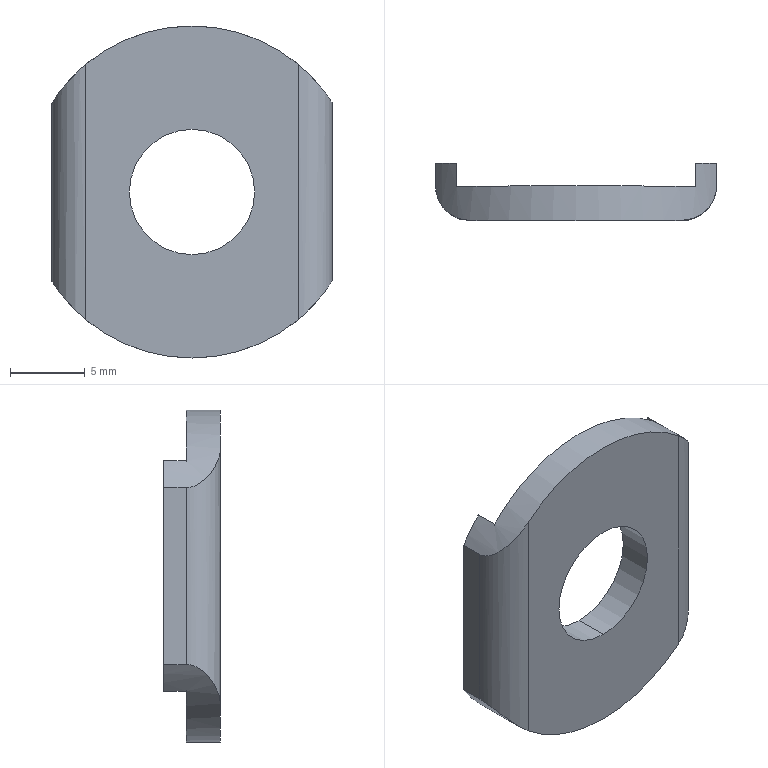Part | SolidWorks | features Boss 1, Cut 1, Extrusion 1, Fillet 1 | 1 solid | 15 faces | box 18.796 x 3.81 x 22.225 mm | volume 726.565 mm3 | plane 8 | cylinder 7 | commonest cylinder face diameters 22.225 x3 4.572 x2 8.382 x2
STEP:
#1=CARTESIAN_POINT('',(0.,0.09,-0.165));
#2=VERTEX_POINT('',#1);
#3=CARTESIAN_POINT('',(0.,0.09,0.165));
#4=VERTEX_POINT('',#3);
#5=CARTESIAN_POINT('',(0.,0.09,0.));
#6=DIRECTION('',(0.,1.,0.));
#7=DIRECTION('',(0.,0.,1.));
#8=AXIS2_PLACEMENT_3D('',#5,#6,#7);
#9=CIRCLE('',#8,0.165);
#10=EDGE_CURVE('',#2,#4,#9,.T.);
#11=ORIENTED_EDGE('',*,*,#10,.T.);
#12=CARTESIAN_POINT('',(0.,0.,0.165));
#13=VERTEX_POINT('',#12);
#14=CARTESIAN_POINT('',(0.,0.09,0.165));
#15=DIRECTION('',(0.,-1.,0.));
#16=VECTOR('',#15,39.37);
#17=LINE('',#14,#16);
#18=EDGE_CURVE('',#4,#13,#17,.T.);
#19=ORIENTED_EDGE('',*,*,#18,.T.);
#20=CARTESIAN_POINT('',(0.,0.,-0.165));
#21=VERTEX_POINT('',#20);
#22=CARTESIAN_POINT('',(0.,0.,0.));
#23=DIRECTION('',(0.,1.,0.));
#24=DIRECTION('',(0.,0.,1.));
#25=AXIS2_PLACEMENT_3D('',#22,#23,#24);
#26=CIRCLE('',#25,0.165);
#27=EDGE_CURVE('',#21,#13,#26,.T.);
#28=ORIENTED_EDGE('',*,*,#27,.F.);
#29=CARTESIAN_POINT('',(0.,0.09,-0.165));
#30=DIRECTION('',(0.,-1.,0.));
#31=VECTOR('',#30,39.37);
#32=LINE('',#29,#31);
#33=EDGE_CURVE('',#2,#21,#32,.T.);
#34=ORIENTED_EDGE('',*,*,#33,.F.);
#35=EDGE_LOOP('',(#11,#19,#28,#34));
#36=FACE_OUTER_BOUND('',#35,.T.);
#37=CARTESIAN_POINT('',(0.,0.09,0.));
#38=DIRECTION('',(0.,-1.,0.));
#39=DIRECTION('',(0.,0.,-1.));
#40=AXIS2_PLACEMENT_3D('',#37,#38,#39);
#41=CYLINDRICAL_SURFACE('',#40,0.165);
#42=ADVANCED_FACE('',(#36),#41,.F.);
#43=CARTESIAN_POINT('',(0.,0.09,-0.4375));
#44=VERTEX_POINT('',#43);
#45=CARTESIAN_POINT('',(-0.315,0.09,-0.3036));
#46=VERTEX_POINT('',#45);
#47=CARTESIAN_POINT('',(0.,0.09,0.));
#48=DIRECTION('',(0.,1.,0.));
#49=DIRECTION('',(0.,0.,1.));
#50=AXIS2_PLACEMENT_3D('',#47,#48,#49);
#51=CIRCLE('',#50,0.4375);
#52=EDGE_CURVE('',#44,#46,#51,.T.);
#53=ORIENTED_EDGE('',*,*,#52,.F.);
#54=CARTESIAN_POINT('',(0.,0.,-0.4375));
#55=VERTEX_POINT('',#54);
#56=CARTESIAN_POINT('',(0.,0.09,-0.4375));
#57=DIRECTION('',(0.,-1.,0.));
#58=VECTOR('',#57,39.37);
#59=LINE('',#56,#58);
#60=EDGE_CURVE('',#44,#55,#59,.T.);
#61=ORIENTED_EDGE('',*,*,#60,.T.);
#62=CARTESIAN_POINT('',(-0.28,0.,-0.3362));
#63=VERTEX_POINT('',#62);
#64=CARTESIAN_POINT('',(0.,0.,0.));
#65=DIRECTION('',(0.,1.,0.));
#66=DIRECTION('',(0.,0.,1.));
#67=AXIS2_PLACEMENT_3D('',#64,#65,#66);
#68=CIRCLE('',#67,0.4375);
#69=EDGE_CURVE('',#55,#63,#68,.T.);
#70=ORIENTED_EDGE('',*,*,#69,.T.);
#71=CARTESIAN_POINT('',(-0.37,0.09,-0.2335));
#72=VERTEX_POINT('',#71);
#73=CARTESIAN_POINT('',(-0.28,0.,-0.3362));
#74=CARTESIAN_POINT('',(-0.2915,0.,-0.3266));
#75=CARTESIAN_POINT('',(-0.3022,0.002115,-0.3167));
#76=CARTESIAN_POINT('',(-0.3223,0.009854,-0.2962));
#77=CARTESIAN_POINT('',(-0.3314,0.01534,-0.2859));
#78=CARTESIAN_POINT('',(-0.3437,0.02614,-0.2708));
#79=CARTESIAN_POINT('',(-0.3475,0.03021,-0.2658));
#80=CARTESIAN_POINT('',(-0.3545,0.03923,-0.2564));
#81=CARTESIAN_POINT('',(-0.3577,0.04421,-0.2519));
#82=CARTESIAN_POINT('',(-0.3633,0.05542,-0.2438));
#83=CARTESIAN_POINT('',(-0.3657,0.06151,-0.2402));
#84=CARTESIAN_POINT('',(-0.369,0.07516,-0.235));
#85=CARTESIAN_POINT('',(-0.37,0.08247,-0.2335));
#86=CARTESIAN_POINT('',(-0.37,0.09,-0.2335));
#87=B_SPLINE_CURVE_WITH_KNOTS('',3,(#73,#74,#75,#76,#77,#78,#79,#80,#81,#82,#83,#84,#85,#86),.UNSPECIFIED.,.F.,.F.,(4,2,2,2,2,2,4),(0.,0.001125,0.00225,0.002813,0.003375,0.003938,0.0045),.UNSPECIFIED.);
#88=EDGE_CURVE('',#63,#72,#87,.T.);
#89=ORIENTED_EDGE('',*,*,#88,.T.);
#90=CARTESIAN_POINT('',(-0.37,0.15,-0.2335));
#91=VERTEX_POINT('',#90);
#92=CARTESIAN_POINT('',(-0.37,0.09,-0.2335));
#93=DIRECTION('',(0.,1.,0.));
#94=VECTOR('',#93,39.37);
#95=LINE('',#92,#94);
#96=EDGE_CURVE('',#72,#91,#95,.T.);
#97=ORIENTED_EDGE('',*,*,#96,.T.);
#98=CARTESIAN_POINT('',(-0.315,0.15,-0.3036));
#99=VERTEX_POINT('',#98);
#100=CARTESIAN_POINT('',(0.,0.15,0.));
#101=DIRECTION('',(0.,1.,0.));
#102=DIRECTION('',(0.,0.,1.));
#103=AXIS2_PLACEMENT_3D('',#100,#101,#102);
#104=CIRCLE('',#103,0.4375);
#105=EDGE_CURVE('',#99,#91,#104,.T.);
#106=ORIENTED_EDGE('',*,*,#105,.F.);
#107=CARTESIAN_POINT('',(-0.315,0.15,-0.3036));
#108=DIRECTION('',(0.,-1.,0.));
#109=VECTOR('',#108,39.37);
#110=LINE('',#107,#109);
#111=EDGE_CURVE('',#99,#46,#110,.T.);
#112=ORIENTED_EDGE('',*,*,#111,.T.);
#113=EDGE_LOOP('',(#53,#61,#70,#89,#97,#106,#112));
#114=FACE_OUTER_BOUND('',#113,.T.);
#115=CARTESIAN_POINT('',(0.,0.09,0.));
#116=DIRECTION('',(0.,-1.,0.));
#117=DIRECTION('',(0.,0.,-1.));
#118=AXIS2_PLACEMENT_3D('',#115,#116,#117);
#119=CYLINDRICAL_SURFACE('',#118,0.4375);
#120=ADVANCED_FACE('',(#114),#119,.T.);
#121=CARTESIAN_POINT('',(0.315,0.09,0.3036));
#122=VERTEX_POINT('',#121);
#123=CARTESIAN_POINT('',(0.315,0.09,-0.3036));
#124=VERTEX_POINT('',#123);
#125=CARTESIAN_POINT('',(0.315,0.09,0.3036));
#126=DIRECTION('',(0.,0.,-1.));
#127=VECTOR('',#126,39.37);
#128=LINE('',#125,#127);
#129=EDGE_CURVE('',#122,#124,#128,.T.);
#130=ORIENTED_EDGE('',*,*,#129,.T.);
#131=CARTESIAN_POINT('',(0.,0.09,0.));
#132=DIRECTION('',(0.,1.,0.));
#133=DIRECTION('',(0.,0.,1.));
#134=AXIS2_PLACEMENT_3D('',#131,#132,#133);
#135=CIRCLE('',#134,0.4375);
#136=EDGE_CURVE('',#124,#44,#135,.T.);
#137=ORIENTED_EDGE('',*,*,#136,.T.);
#138=ORIENTED_EDGE('',*,*,#52,.T.);
#139=CARTESIAN_POINT('',(-0.315,0.09,0.3036));
#140=VERTEX_POINT('',#139);
#141=CARTESIAN_POINT('',(-0.315,0.09,-0.3036));
#142=DIRECTION('',(0.,0.,1.));
#143=VECTOR('',#142,39.37);
#144=LINE('',#141,#143);
#145=EDGE_CURVE('',#46,#140,#144,.T.);
#146=ORIENTED_EDGE('',*,*,#145,.T.);
#147=CARTESIAN_POINT('',(0.,0.09,0.));
#148=DIRECTION('',(0.,1.,0.));
#149=DIRECTION('',(0.,0.,1.));
#150=AXIS2_PLACEMENT_3D('',#147,#148,#149);
#151=CIRCLE('',#150,0.4375);
#152=EDGE_CURVE('',#140,#122,#151,.T.);
#153=ORIENTED_EDGE('',*,*,#152,.T.);
#154=EDGE_LOOP('',(#130,#137,#138,#146,#153));
#155=FACE_OUTER_BOUND('',#154,.T.);
#156=ORIENTED_EDGE('',*,*,#10,.F.);
#157=CARTESIAN_POINT('',(0.,0.09,0.));
#158=DIRECTION('',(0.,1.,0.));
#159=DIRECTION('',(0.,0.,1.));
#160=AXIS2_PLACEMENT_3D('',#157,#158,#159);
#161=CIRCLE('',#160,0.165);
#162=EDGE_CURVE('',#4,#2,#161,.T.);
#163=ORIENTED_EDGE('',*,*,#162,.F.);
#164=EDGE_LOOP('',(#156,#163));
#165=FACE_BOUND('',#164,.T.);
#166=CARTESIAN_POINT('',(0.,0.09,0.));
#167=DIRECTION('',(0.,1.,0.));
#168=DIRECTION('',(0.,0.,1.));
#169=AXIS2_PLACEMENT_3D('',#166,#167,#168);
#170=PLANE('',#169);
#171=ADVANCED_FACE('',(#155,#165),#170,.T.);
#172=ORIENTED_EDGE('',*,*,#27,.T.);
#173=CARTESIAN_POINT('',(0.,0.,0.));
#174=DIRECTION('',(0.,1.,0.));
#175=DIRECTION('',(0.,0.,1.));
#176=AXIS2_PLACEMENT_3D('',#173,#174,#175);
#177=CIRCLE('',#176,0.165);
#178=EDGE_CURVE('',#13,#21,#177,.T.);
#179=ORIENTED_EDGE('',*,*,#178,.T.);
#180=EDGE_LOOP('',(#172,#179));
#181=FACE_BOUND('',#180,.T.);
#182=CARTESIAN_POINT('',(-0.28,0.,0.3362));
#183=VERTEX_POINT('',#182);
#184=CARTESIAN_POINT('',(0.28,0.,0.3362));
#185=VERTEX_POINT('',#184);
#186=CARTESIAN_POINT('',(0.,0.,0.));
#187=DIRECTION('',(0.,1.,0.));
#188=DIRECTION('',(0.,0.,1.));
#189=AXIS2_PLACEMENT_3D('',#186,#187,#188);
#190=CIRCLE('',#189,0.4375);
#191=EDGE_CURVE('',#183,#185,#190,.T.);
#192=ORIENTED_EDGE('',*,*,#191,.F.);
#193=CARTESIAN_POINT('',(-0.28,0.,0.));
#194=DIRECTION('',(0.,0.,-1.));
#195=VECTOR('',#194,39.37);
#196=LINE('',#193,#195);
#197=EDGE_CURVE('',#183,#63,#196,.T.);
#198=ORIENTED_EDGE('',*,*,#197,.T.);
#199=ORIENTED_EDGE('',*,*,#69,.F.);
#200=CARTESIAN_POINT('',(0.28,0.,-0.3362));
#201=VERTEX_POINT('',#200);
#202=CARTESIAN_POINT('',(0.,0.,0.));
#203=DIRECTION('',(0.,1.,0.));
#204=DIRECTION('',(0.,0.,1.));
#205=AXIS2_PLACEMENT_3D('',#202,#203,#204);
#206=CIRCLE('',#205,0.4375);
#207=EDGE_CURVE('',#201,#55,#206,.T.);
#208=ORIENTED_EDGE('',*,*,#207,.F.);
#209=CARTESIAN_POINT('',(0.28,0.,0.2335));
#210=DIRECTION('',(0.,0.,1.));
#211=VECTOR('',#210,39.37);
#212=LINE('',#209,#211);
#213=EDGE_CURVE('',#201,#185,#212,.T.);
#214=ORIENTED_EDGE('',*,*,#213,.T.);
#215=EDGE_LOOP('',(#192,#198,#199,#208,#214));
#216=FACE_OUTER_BOUND('',#215,.T.);
#217=CARTESIAN_POINT('',(0.,0.,0.));
#218=DIRECTION('',(0.,1.,0.));
#219=DIRECTION('',(0.,0.,1.));
#220=AXIS2_PLACEMENT_3D('',#217,#218,#219);
#221=PLANE('',#220);
#222=ADVANCED_FACE('',(#181,#216),#221,.F.);
#223=CARTESIAN_POINT('',(-0.37,0.15,0.2335));
#224=VERTEX_POINT('',#223);
#225=CARTESIAN_POINT('',(-0.37,0.09,0.2335));
#226=VERTEX_POINT('',#225);
#227=CARTESIAN_POINT('',(-0.37,0.09,0.2335));
#228=DIRECTION('',(0.,-1.,0.));
#229=VECTOR('',#228,39.37);
#230=LINE('',#227,#229);
#231=EDGE_CURVE('',#224,#226,#230,.T.);
#232=ORIENTED_EDGE('',*,*,#231,.T.);
#233=CARTESIAN_POINT('',(-0.37,0.09,0.2335));
#234=CARTESIAN_POINT('',(-0.37,0.08623,0.2335));
#235=CARTESIAN_POINT('',(-0.3698,0.08254,0.2338));
#236=CARTESIAN_POINT('',(-0.3689,0.07529,0.2353));
#237=CARTESIAN_POINT('',(-0.3682,0.07171,0.2363));
#238=CARTESIAN_POINT('',(-0.3657,0.06155,0.2402));
#239=CARTESIAN_POINT('',(-0.3633,0.05537,0.2438));
#240=CARTESIAN_POINT('',(-0.3577,0.0442,0.2519));
#241=CARTESIAN_POINT('',(-0.3545,0.03924,0.2564));
#242=CARTESIAN_POINT('',(-0.3475,0.03021,0.2658));
#243=CARTESIAN_POINT('',(-0.3437,0.02614,0.2708));
#244=CARTESIAN_POINT('',(-0.3314,0.01536,0.2859));
#245=CARTESIAN_POINT('',(-0.3223,0.009848,0.2962));
#246=CARTESIAN_POINT('',(-0.3022,0.002118,0.3167));
#247=CARTESIAN_POINT('',(-0.2915,0.,0.3266));
#248=CARTESIAN_POINT('',(-0.28,0.,0.3362));
#249=B_SPLINE_CURVE_WITH_KNOTS('',3,(#233,#234,#235,#236,#237,#238,#239,#240,#241,#242,#243,#244,#245,#246,#247,#248),.UNSPECIFIED.,.F.,.F.,(4,2,2,2,2,2,2,4),(0.,0.0002829,0.0005657,0.001131,0.001697,0.002263,0.003394,0.004526),.UNSPECIFIED.);
#250=EDGE_CURVE('',#226,#183,#249,.T.);
#251=ORIENTED_EDGE('',*,*,#250,.T.);
#252=ORIENTED_EDGE('',*,*,#191,.T.);
#253=CARTESIAN_POINT('',(0.37,0.09,0.2335));
#254=VERTEX_POINT('',#253);
#255=CARTESIAN_POINT('',(0.28,0.,0.3362));
#256=CARTESIAN_POINT('',(0.2915,0.,0.3266));
#257=CARTESIAN_POINT('',(0.3022,0.002115,0.3167));
#258=CARTESIAN_POINT('',(0.3223,0.009854,0.2962));
#259=CARTESIAN_POINT('',(0.3314,0.01534,0.2859));
#260=CARTESIAN_POINT('',(0.3437,0.02614,0.2708));
#261=CARTESIAN_POINT('',(0.3475,0.03021,0.2658));
#262=CARTESIAN_POINT('',(0.3545,0.03923,0.2564));
#263=CARTESIAN_POINT('',(0.3577,0.04421,0.2519));
#264=CARTESIAN_POINT('',(0.3633,0.05542,0.2438));
#265=CARTESIAN_POINT('',(0.3657,0.06151,0.2402));
#266=CARTESIAN_POINT('',(0.369,0.07516,0.235));
#267=CARTESIAN_POINT('',(0.37,0.08247,0.2335));
#268=CARTESIAN_POINT('',(0.37,0.09,0.2335));
#269=B_SPLINE_CURVE_WITH_KNOTS('',3,(#255,#256,#257,#258,#259,#260,#261,#262,#263,#264,#265,#266,#267,#268),.UNSPECIFIED.,.F.,.F.,(4,2,2,2,2,2,4),(0.,0.001125,0.00225,0.002813,0.003375,0.003938,0.0045),.UNSPECIFIED.);
#270=EDGE_CURVE('',#185,#254,#269,.T.);
#271=ORIENTED_EDGE('',*,*,#270,.T.);
#272=CARTESIAN_POINT('',(0.37,0.15,0.2335));
#273=VERTEX_POINT('',#272);
#274=CARTESIAN_POINT('',(0.37,0.09,0.2335));
#275=DIRECTION('',(0.,-1.,0.));
#276=VECTOR('',#275,39.37);
#277=LINE('',#274,#276);
#278=EDGE_CURVE('',#273,#254,#277,.T.);
#279=ORIENTED_EDGE('',*,*,#278,.F.);
#280=CARTESIAN_POINT('',(0.315,0.15,0.3036));
#281=VERTEX_POINT('',#280);
#282=CARTESIAN_POINT('',(0.,0.15,0.));
#283=DIRECTION('',(0.,1.,0.));
#284=DIRECTION('',(0.,0.,1.));
#285=AXIS2_PLACEMENT_3D('',#282,#283,#284);
#286=CIRCLE('',#285,0.4375);
#287=EDGE_CURVE('',#281,#273,#286,.T.);
#288=ORIENTED_EDGE('',*,*,#287,.F.);
#289=CARTESIAN_POINT('',(0.315,0.15,0.3036));
#290=DIRECTION('',(0.,-1.,0.));
#291=VECTOR('',#290,39.37);
#292=LINE('',#289,#291);
#293=EDGE_CURVE('',#281,#122,#292,.T.);
#294=ORIENTED_EDGE('',*,*,#293,.T.);
#295=ORIENTED_EDGE('',*,*,#152,.F.);
#296=CARTESIAN_POINT('',(-0.315,0.15,0.3036));
#297=VERTEX_POINT('',#296);
#298=CARTESIAN_POINT('',(-0.315,0.15,0.3036));
#299=DIRECTION('',(0.,-1.,0.));
#300=VECTOR('',#299,39.37);
#301=LINE('',#298,#300);
#302=EDGE_CURVE('',#297,#140,#301,.T.);
#303=ORIENTED_EDGE('',*,*,#302,.F.);
#304=CARTESIAN_POINT('',(0.,0.15,0.));
#305=DIRECTION('',(0.,1.,0.));
#306=DIRECTION('',(0.,0.,1.));
#307=AXIS2_PLACEMENT_3D('',#304,#305,#306);
#308=CIRCLE('',#307,0.4375);
#309=EDGE_CURVE('',#224,#297,#308,.T.);
#310=ORIENTED_EDGE('',*,*,#309,.F.);
#311=EDGE_LOOP('',(#232,#251,#252,#271,#279,#288,#294,#295,#303,#310));
#312=FACE_OUTER_BOUND('',#311,.T.);
#313=CARTESIAN_POINT('',(0.,0.09,0.));
#314=DIRECTION('',(0.,-1.,0.));
#315=DIRECTION('',(0.,0.,-1.));
#316=AXIS2_PLACEMENT_3D('',#313,#314,#315);
#317=CYLINDRICAL_SURFACE('',#316,0.4375);
#318=ADVANCED_FACE('',(#312),#317,.T.);
#319=ORIENTED_EDGE('',*,*,#60,.F.);
#320=ORIENTED_EDGE('',*,*,#136,.F.);
#321=CARTESIAN_POINT('',(0.315,0.15,-0.3036));
#322=VERTEX_POINT('',#321);
#323=CARTESIAN_POINT('',(0.315,0.15,-0.3036));
#324=DIRECTION('',(0.,-1.,0.));
#325=VECTOR('',#324,39.37);
#326=LINE('',#323,#325);
#327=EDGE_CURVE('',#322,#124,#326,.T.);
#328=ORIENTED_EDGE('',*,*,#327,.F.);
#329=CARTESIAN_POINT('',(0.37,0.15,-0.2335));
#330=VERTEX_POINT('',#329);
#331=CARTESIAN_POINT('',(0.,0.15,0.));
#332=DIRECTION('',(0.,1.,0.));
#333=DIRECTION('',(0.,0.,1.));
#334=AXIS2_PLACEMENT_3D('',#331,#332,#333);
#335=CIRCLE('',#334,0.4375);
#336=EDGE_CURVE('',#330,#322,#335,.T.);
#337=ORIENTED_EDGE('',*,*,#336,.F.);
#338=CARTESIAN_POINT('',(0.37,0.09,-0.2335));
#339=VERTEX_POINT('',#338);
#340=CARTESIAN_POINT('',(0.37,0.09,-0.2335));
#341=DIRECTION('',(0.,1.,0.));
#342=VECTOR('',#341,39.37);
#343=LINE('',#340,#342);
#344=EDGE_CURVE('',#339,#330,#343,.T.);
#345=ORIENTED_EDGE('',*,*,#344,.F.);
#346=CARTESIAN_POINT('',(0.37,0.09,-0.2335));
#347=CARTESIAN_POINT('',(0.37,0.08623,-0.2335));
#348=CARTESIAN_POINT('',(0.3698,0.08254,-0.2338));
#349=CARTESIAN_POINT('',(0.3689,0.07529,-0.2353));
#350=CARTESIAN_POINT('',(0.3682,0.07171,-0.2363));
#351=CARTESIAN_POINT('',(0.3657,0.06155,-0.2402));
#352=CARTESIAN_POINT('',(0.3633,0.05537,-0.2438));
#353=CARTESIAN_POINT('',(0.3577,0.0442,-0.2519));
#354=CARTESIAN_POINT('',(0.3545,0.03924,-0.2564));
#355=CARTESIAN_POINT('',(0.3475,0.03021,-0.2658));
#356=CARTESIAN_POINT('',(0.3437,0.02614,-0.2708));
#357=CARTESIAN_POINT('',(0.3314,0.01536,-0.2859));
#358=CARTESIAN_POINT('',(0.3223,0.009848,-0.2962));
#359=CARTESIAN_POINT('',(0.3022,0.002118,-0.3167));
#360=CARTESIAN_POINT('',(0.2915,0.,-0.3266));
#361=CARTESIAN_POINT('',(0.28,0.,-0.3362));
#362=B_SPLINE_CURVE_WITH_KNOTS('',3,(#346,#347,#348,#349,#350,#351,#352,#353,#354,#355,#356,#357,#358,#359,#360,#361),.UNSPECIFIED.,.F.,.F.,(4,2,2,2,2,2,2,4),(0.,0.0002829,0.0005657,0.001131,0.001697,0.002263,0.003394,0.004526),.UNSPECIFIED.);
#363=EDGE_CURVE('',#339,#201,#362,.T.);
#364=ORIENTED_EDGE('',*,*,#363,.T.);
#365=ORIENTED_EDGE('',*,*,#207,.T.);
#366=EDGE_LOOP('',(#319,#320,#328,#337,#345,#364,#365));
#367=FACE_OUTER_BOUND('',#366,.T.);
#368=CARTESIAN_POINT('',(0.,0.09,0.));
#369=DIRECTION('',(0.,-1.,0.));
#370=DIRECTION('',(0.,0.,-1.));
#371=AXIS2_PLACEMENT_3D('',#368,#369,#370);
#372=CYLINDRICAL_SURFACE('',#371,0.4375);
#373=ADVANCED_FACE('',(#367),#372,.T.);
#374=ORIENTED_EDGE('',*,*,#18,.F.);
#375=ORIENTED_EDGE('',*,*,#162,.T.);
#376=ORIENTED_EDGE('',*,*,#33,.T.);
#377=ORIENTED_EDGE('',*,*,#178,.F.);
#378=EDGE_LOOP('',(#374,#375,#376,#377));
#379=FACE_OUTER_BOUND('',#378,.T.);
#380=CARTESIAN_POINT('',(0.,0.09,0.));
#381=DIRECTION('',(0.,-1.,0.));
#382=DIRECTION('',(0.,0.,-1.));
#383=AXIS2_PLACEMENT_3D('',#380,#381,#382);
#384=CYLINDRICAL_SURFACE('',#383,0.165);
#385=ADVANCED_FACE('',(#379),#384,.F.);
#386=ORIENTED_EDGE('',*,*,#278,.T.);
#387=CARTESIAN_POINT('',(0.37,0.09,-0.2335));
#388=DIRECTION('',(0.,0.,-1.));
#389=VECTOR('',#388,39.37);
#390=LINE('',#387,#389);
#391=EDGE_CURVE('',#254,#339,#390,.T.);
#392=ORIENTED_EDGE('',*,*,#391,.T.);
#393=ORIENTED_EDGE('',*,*,#344,.T.);
#394=CARTESIAN_POINT('',(0.37,0.15,0.2335));
#395=DIRECTION('',(0.,0.,-1.));
#396=VECTOR('',#395,39.37);
#397=LINE('',#394,#396);
#398=EDGE_CURVE('',#273,#330,#397,.T.);
#399=ORIENTED_EDGE('',*,*,#398,.F.);
#400=EDGE_LOOP('',(#386,#392,#393,#399));
#401=FACE_OUTER_BOUND('',#400,.T.);
#402=CARTESIAN_POINT('',(0.37,0.09,-0.3948));
#403=DIRECTION('',(1.,0.,0.));
#404=DIRECTION('',(0.,0.,-1.));
#405=AXIS2_PLACEMENT_3D('',#402,#403,#404);
#406=PLANE('',#405);
#407=ADVANCED_FACE('',(#401),#406,.T.);
#408=ORIENTED_EDGE('',*,*,#96,.F.);
#409=CARTESIAN_POINT('',(-0.37,0.09,-0.3948));
#410=DIRECTION('',(0.,0.,1.));
#411=VECTOR('',#410,39.37);
#412=LINE('',#409,#411);
#413=EDGE_CURVE('',#72,#226,#412,.T.);
#414=ORIENTED_EDGE('',*,*,#413,.T.);
#415=ORIENTED_EDGE('',*,*,#231,.F.);
#416=CARTESIAN_POINT('',(-0.37,0.15,-0.2335));
#417=DIRECTION('',(0.,0.,1.));
#418=VECTOR('',#417,39.37);
#419=LINE('',#416,#418);
#420=EDGE_CURVE('',#91,#224,#419,.T.);
#421=ORIENTED_EDGE('',*,*,#420,.F.);
#422=EDGE_LOOP('',(#408,#414,#415,#421));
#423=FACE_OUTER_BOUND('',#422,.T.);
#424=CARTESIAN_POINT('',(-0.37,0.09,-0.3948));
#425=DIRECTION('',(1.,0.,0.));
#426=DIRECTION('',(0.,0.,-1.));
#427=AXIS2_PLACEMENT_3D('',#424,#425,#426);
#428=PLANE('',#427);
#429=ADVANCED_FACE('',(#423),#428,.F.);
#430=ORIENTED_EDGE('',*,*,#145,.F.);
#431=ORIENTED_EDGE('',*,*,#111,.F.);
#432=CARTESIAN_POINT('',(-0.315,0.15,-0.3036));
#433=DIRECTION('',(0.,0.,1.));
#434=VECTOR('',#433,39.37);
#435=LINE('',#432,#434);
#436=EDGE_CURVE('',#99,#297,#435,.T.);
#437=ORIENTED_EDGE('',*,*,#436,.T.);
#438=ORIENTED_EDGE('',*,*,#302,.T.);
#439=EDGE_LOOP('',(#430,#431,#437,#438));
#440=FACE_OUTER_BOUND('',#439,.T.);
#441=CARTESIAN_POINT('',(-0.315,0.15,-0.3036));
#442=DIRECTION('',(1.,0.,0.));
#443=DIRECTION('',(0.,0.,-1.));
#444=AXIS2_PLACEMENT_3D('',#441,#442,#443);
#445=PLANE('',#444);
#446=ADVANCED_FACE('',(#440),#445,.T.);
#447=ORIENTED_EDGE('',*,*,#105,.T.);
#448=ORIENTED_EDGE('',*,*,#420,.T.);
#449=ORIENTED_EDGE('',*,*,#309,.T.);
#450=ORIENTED_EDGE('',*,*,#436,.F.);
#451=EDGE_LOOP('',(#447,#448,#449,#450));
#452=FACE_OUTER_BOUND('',#451,.T.);
#453=CARTESIAN_POINT('',(0.,0.15,0.));
#454=DIRECTION('',(0.,1.,0.));
#455=DIRECTION('',(0.,0.,1.));
#456=AXIS2_PLACEMENT_3D('',#453,#454,#455);
#457=PLANE('',#456);
#458=ADVANCED_FACE('',(#452),#457,.T.);
#459=ORIENTED_EDGE('',*,*,#129,.F.);
#460=ORIENTED_EDGE('',*,*,#293,.F.);
#461=CARTESIAN_POINT('',(0.315,0.15,0.3036));
#462=DIRECTION('',(0.,0.,-1.));
#463=VECTOR('',#462,39.37);
#464=LINE('',#461,#463);
#465=EDGE_CURVE('',#281,#322,#464,.T.);
#466=ORIENTED_EDGE('',*,*,#465,.T.);
#467=ORIENTED_EDGE('',*,*,#327,.T.);
#468=EDGE_LOOP('',(#459,#460,#466,#467));
#469=FACE_OUTER_BOUND('',#468,.T.);
#470=CARTESIAN_POINT('',(0.315,0.15,0.3036));
#471=DIRECTION('',(-1.,0.,0.));
#472=DIRECTION('',(0.,0.,1.));
#473=AXIS2_PLACEMENT_3D('',#470,#471,#472);
#474=PLANE('',#473);
#475=ADVANCED_FACE('',(#469),#474,.T.);
#476=ORIENTED_EDGE('',*,*,#287,.T.);
#477=ORIENTED_EDGE('',*,*,#398,.T.);
#478=ORIENTED_EDGE('',*,*,#336,.T.);
#479=ORIENTED_EDGE('',*,*,#465,.F.);
#480=EDGE_LOOP('',(#476,#477,#478,#479));
#481=FACE_OUTER_BOUND('',#480,.T.);
#482=CARTESIAN_POINT('',(0.,0.15,0.));
#483=DIRECTION('',(0.,1.,0.));
#484=DIRECTION('',(0.,0.,1.));
#485=AXIS2_PLACEMENT_3D('',#482,#483,#484);
#486=PLANE('',#485);
#487=ADVANCED_FACE('',(#481),#486,.T.);
#488=ORIENTED_EDGE('',*,*,#250,.F.);
#489=ORIENTED_EDGE('',*,*,#413,.F.);
#490=ORIENTED_EDGE('',*,*,#88,.F.);
#491=ORIENTED_EDGE('',*,*,#197,.F.);
#492=EDGE_LOOP('',(#488,#489,#490,#491));
#493=FACE_OUTER_BOUND('',#492,.T.);
#494=CARTESIAN_POINT('',(-0.28,0.09,0.));
#495=DIRECTION('',(0.,0.,-1.));
#496=DIRECTION('',(-1.,0.,0.));
#497=AXIS2_PLACEMENT_3D('',#494,#495,#496);
#498=CYLINDRICAL_SURFACE('',#497,0.09);
#499=ADVANCED_FACE('',(#493),#498,.T.);
#500=ORIENTED_EDGE('',*,*,#270,.F.);
#501=ORIENTED_EDGE('',*,*,#213,.F.);
#502=ORIENTED_EDGE('',*,*,#363,.F.);
#503=ORIENTED_EDGE('',*,*,#391,.F.);
#504=EDGE_LOOP('',(#500,#501,#502,#503));
#505=FACE_OUTER_BOUND('',#504,.T.);
#506=CARTESIAN_POINT('',(0.28,0.09,-0.3948));
#507=DIRECTION('',(0.,0.,1.));
#508=DIRECTION('',(1.,0.,0.));
#509=AXIS2_PLACEMENT_3D('',#506,#507,#508);
#510=CYLINDRICAL_SURFACE('',#509,0.09);
#511=ADVANCED_FACE('',(#505),#510,.T.);
#512=CLOSED_SHELL('',(#42,#120,#171,#222,#318,#373,#385,#407,#429,#446,#458,#475,#487,#499,#511));
#513=MANIFOLD_SOLID_BREP('',#512);
#514=CARTESIAN_POINT('',(0.,0.,0.));
#515=DIRECTION('',(0.,0.,1.));
#516=DIRECTION('',(1.,0.,0.));
#517=AXIS2_PLACEMENT_3D('',#514,#515,#516);
#518=(LENGTH_UNIT()NAMED_UNIT(*)SI_UNIT($,.METRE.));
#519=LENGTH_MEASURE_WITH_UNIT(LENGTH_MEASURE(0.0254),#518);
#520=DIMENSIONAL_EXPONENTS(1.,0.,0.,0.,0.,0.,0.);
#521=(CONVERSION_BASED_UNIT('INCH',#519)LENGTH_UNIT()NAMED_UNIT(#520));
#522=UNCERTAINTY_MEASURE_WITH_UNIT(LENGTH_MEASURE(0.00001),#521,'','');
#523=(NAMED_UNIT(*)PLANE_ANGLE_UNIT()SI_UNIT($,.RADIAN.));
#524=(NAMED_UNIT(*)SI_UNIT($,.STERADIAN.)SOLID_ANGLE_UNIT());
#525=(GEOMETRIC_REPRESENTATION_CONTEXT(3)GLOBAL_UNCERTAINTY_ASSIGNED_CONTEXT((#522))GLOBAL_UNIT_ASSIGNED_CONTEXT((#521,#523,#524))REPRESENTATION_CONTEXT('',''));
#526=ADVANCED_BREP_SHAPE_REPRESENTATION('',(#513,#517),#525);